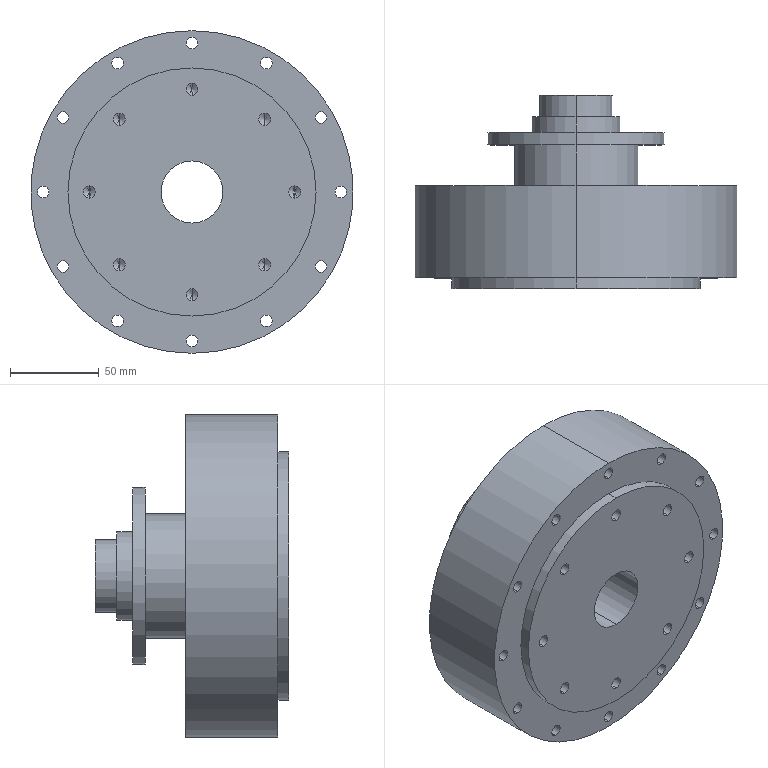Part | SolidWorks | features HoleWzd 2, ICE 1, RevCut 1, Revolution 1 | 1 solid | 77 faces | box 182 x 109 x 182 mm | volume 1490023 mm3 | cylinder 54 | cone 16 | plane 7 | commonest cylinder face diameters 6.6 x24 6.8 x16 35 x2 41 x2 50 x2 70 x2